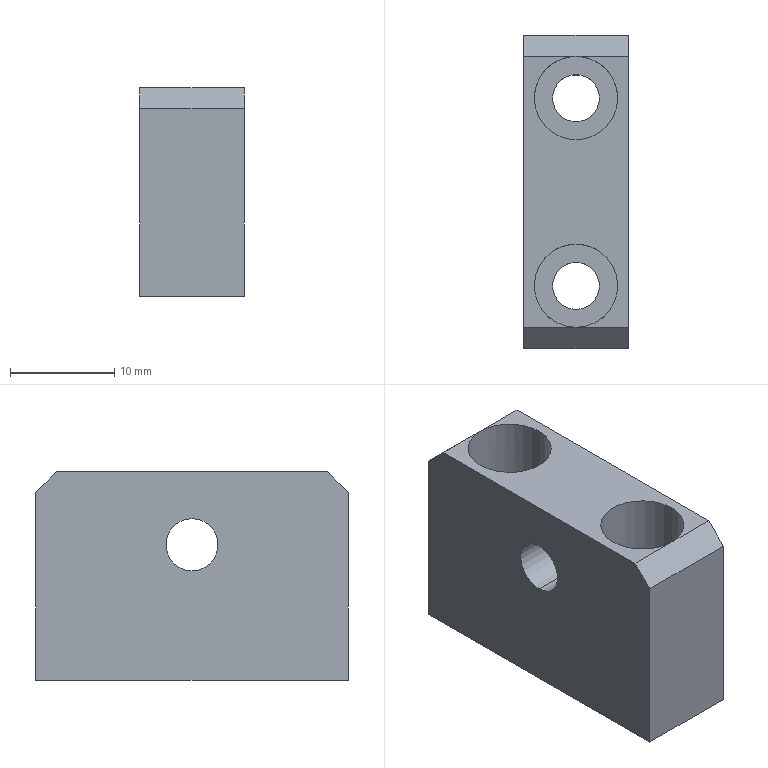Part | STEP file | PN_0030 | 1 solid | 20 faces | box 10 x 30 x 20 mm | volume 4165 mm3 | cylinder 10 | plane 10 | commonest cylinder face diameters 4.5 x4 8 x4 5 x2